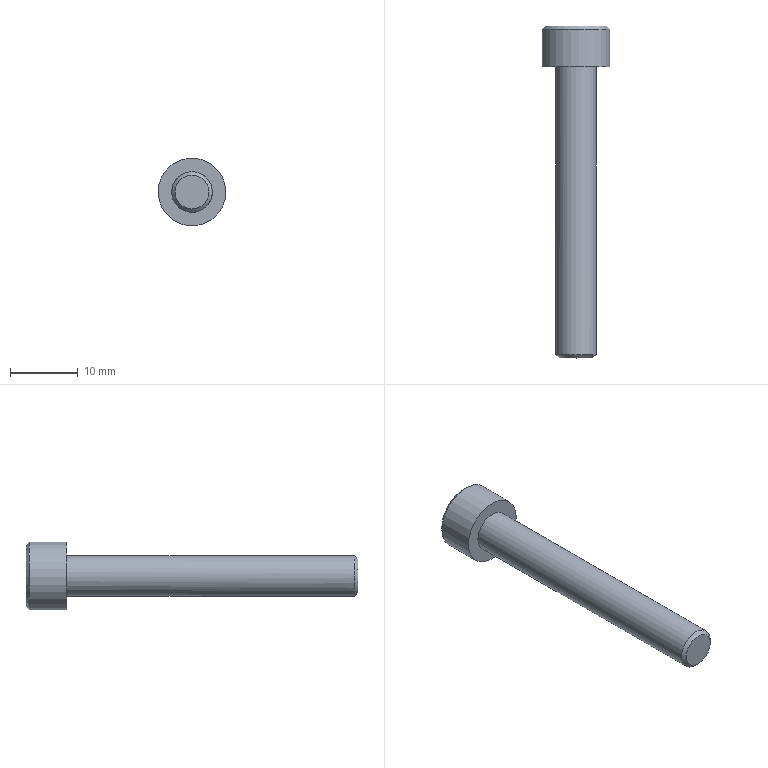Part | NX | features 切除-拉伸1 2 | 1 solid | 20 faces | box 10 x 49 x 10 mm | volume 1607 mm3 | plane 15 | cone 3 | cylinder 2 | commonest cylinder face diameters 6 x1 10 x1
STEP:
#1=CARTESIAN_POINT('',(17.5,309.216,107.881));
#2=VERTEX_POINT('',#1);
#3=CARTESIAN_POINT('',(17.5,309.216,105.381));
#4=DIRECTION('',(0.,1.,0.));
#5=DIRECTION('',(0.,0.,1.));
#6=AXIS2_PLACEMENT_3D('',#3,#4,#5);
#7=CIRCLE('',#6,2.5);
#8=EDGE_CURVE('',#2,#2,#7,.F.);
#9=ORIENTED_EDGE('',*,*,#8,.T.);
#10=EDGE_LOOP('',(#9));
#11=FACE_BOUND('',#10,.T.);
#12=CARTESIAN_POINT('',(-17.5,309.216,105.381));
#13=DIRECTION('',(0.,1.,0.));
#14=DIRECTION('',(-0.07719,0.,0.997));
#15=AXIS2_PLACEMENT_3D('',#12,#13,#14);
#16=PLANE('',#15);
#17=ADVANCED_FACE('',(#11),#16,.F.);
#18=CARTESIAN_POINT('',(17.5,309.716,108.381));
#19=VERTEX_POINT('',#18);
#20=CARTESIAN_POINT('',(17.5,309.716,105.381));
#21=DIRECTION('',(0.,1.,0.));
#22=DIRECTION('',(0.,0.,1.));
#23=AXIS2_PLACEMENT_3D('',#20,#21,#22);
#24=CIRCLE('',#23,3.);
#25=EDGE_CURVE('',#19,#19,#24,.T.);
#26=ORIENTED_EDGE('',*,*,#25,.T.);
#27=EDGE_LOOP('',(#26));
#28=FACE_BOUND('',#27,.T.);
#29=CARTESIAN_POINT('',(14.603,352.216,104.603));
#30=VERTEX_POINT('',#29);
#31=CARTESIAN_POINT('',(17.5,352.216,105.381));
#32=DIRECTION('',(0.,1.,0.));
#33=DIRECTION('',(-0.9657,0.,-0.2595));
#34=AXIS2_PLACEMENT_3D('',#31,#32,#33);
#35=CIRCLE('',#34,3.);
#36=EDGE_CURVE('',#30,#30,#35,.T.);
#37=ORIENTED_EDGE('',*,*,#36,.F.);
#38=EDGE_LOOP('',(#37));
#39=FACE_BOUND('',#38,.T.);
#40=CARTESIAN_POINT('',(17.5,359.966,105.381));
#41=DIRECTION('',(0.,1.,0.));
#42=DIRECTION('',(0.9657,0.,0.2595));
#43=AXIS2_PLACEMENT_3D('',#40,#41,#42);
#44=CYLINDRICAL_SURFACE('',#43,3.);
#45=ADVANCED_FACE('',(#28,#39),#44,.T.);
#46=CARTESIAN_POINT('',(16.855,355.216,102.966));
#47=VERTEX_POINT('',#46);
#48=CARTESIAN_POINT('',(15.086,355.216,104.732));
#49=VERTEX_POINT('',#48);
#50=CARTESIAN_POINT('',(17.5,355.216,105.381));
#51=DIRECTION('',(0.,1.,0.));
#52=DIRECTION('',(-0.9657,0.,-0.2595));
#53=AXIS2_PLACEMENT_3D('',#50,#51,#52);
#54=CIRCLE('',#53,2.5);
#55=EDGE_CURVE('',#47,#49,#54,.T.);
#56=ORIENTED_EDGE('',*,*,#55,.T.);
#57=CARTESIAN_POINT('',(15.731,355.216,107.148));
#58=VERTEX_POINT('',#57);
#59=CARTESIAN_POINT('',(17.5,355.216,105.381));
#60=DIRECTION('',(0.,1.,0.));
#61=DIRECTION('',(-0.9657,0.,-0.2595));
#62=AXIS2_PLACEMENT_3D('',#59,#60,#61);
#63=CIRCLE('',#62,2.5);
#64=EDGE_CURVE('',#49,#58,#63,.T.);
#65=ORIENTED_EDGE('',*,*,#64,.T.);
#66=CARTESIAN_POINT('',(18.145,355.216,107.797));
#67=VERTEX_POINT('',#66);
#68=CARTESIAN_POINT('',(17.5,355.216,105.381));
#69=DIRECTION('',(0.,1.,0.));
#70=DIRECTION('',(-0.9657,0.,-0.2595));
#71=AXIS2_PLACEMENT_3D('',#68,#69,#70);
#72=CIRCLE('',#71,2.5);
#73=EDGE_CURVE('',#58,#67,#72,.T.);
#74=ORIENTED_EDGE('',*,*,#73,.T.);
#75=CARTESIAN_POINT('',(19.914,355.216,106.03));
#76=VERTEX_POINT('',#75);
#77=CARTESIAN_POINT('',(17.5,355.216,105.381));
#78=DIRECTION('',(0.,1.,0.));
#79=DIRECTION('',(-0.9657,0.,-0.2595));
#80=AXIS2_PLACEMENT_3D('',#77,#78,#79);
#81=CIRCLE('',#80,2.5);
#82=EDGE_CURVE('',#67,#76,#81,.T.);
#83=ORIENTED_EDGE('',*,*,#82,.T.);
#84=CARTESIAN_POINT('',(19.269,355.216,103.615));
#85=VERTEX_POINT('',#84);
#86=CARTESIAN_POINT('',(17.5,355.216,105.381));
#87=DIRECTION('',(0.,1.,0.));
#88=DIRECTION('',(-0.9657,0.,-0.2595));
#89=AXIS2_PLACEMENT_3D('',#86,#87,#88);
#90=CIRCLE('',#89,2.5);
#91=EDGE_CURVE('',#76,#85,#90,.T.);
#92=ORIENTED_EDGE('',*,*,#91,.T.);
#93=CARTESIAN_POINT('',(17.5,355.216,105.381));
#94=DIRECTION('',(0.,1.,0.));
#95=DIRECTION('',(-0.9657,0.,-0.2595));
#96=AXIS2_PLACEMENT_3D('',#93,#94,#95);
#97=CIRCLE('',#96,2.5);
#98=EDGE_CURVE('',#85,#47,#97,.T.);
#99=ORIENTED_EDGE('',*,*,#98,.T.);
#100=EDGE_LOOP('',(#56,#65,#74,#83,#92,#99));
#101=FACE_BOUND('',#100,.T.);
#102=CARTESIAN_POINT('',(17.5,353.772,105.381));
#103=VERTEX_POINT('',#102);
#104=VERTEX_LOOP('',#103);
#105=FACE_BOUND('',#104,.T.);
#106=CARTESIAN_POINT('',(17.5,355.216,105.381));
#107=DIRECTION('',(0.,1.,0.));
#108=DIRECTION('',(0.9657,0.,0.2595));
#109=AXIS2_PLACEMENT_3D('',#106,#107,#108);
#110=CONICAL_SURFACE('',#109,2.5,1.047);
#111=ADVANCED_FACE('',(#101,#105),#110,.F.);
#112=CARTESIAN_POINT('',(22.329,357.736,106.679));
#113=VERTEX_POINT('',#112);
#114=CARTESIAN_POINT('',(17.5,357.736,105.381));
#115=DIRECTION('',(0.,-1.,0.));
#116=DIRECTION('',(0.9657,0.,0.2595));
#117=AXIS2_PLACEMENT_3D('',#114,#115,#116);
#118=CIRCLE('',#117,5.);
#119=EDGE_CURVE('',#113,#113,#118,.T.);
#120=ORIENTED_EDGE('',*,*,#119,.F.);
#121=EDGE_LOOP('',(#120));
#122=FACE_BOUND('',#121,.T.);
#123=CARTESIAN_POINT('',(21.865,358.216,106.554));
#124=VERTEX_POINT('',#123);
#125=CARTESIAN_POINT('',(17.5,358.216,105.381));
#126=DIRECTION('',(0.,1.,0.));
#127=DIRECTION('',(0.9657,0.,0.2595));
#128=AXIS2_PLACEMENT_3D('',#125,#126,#127);
#129=CIRCLE('',#128,4.52);
#130=EDGE_CURVE('',#124,#124,#129,.T.);
#131=ORIENTED_EDGE('',*,*,#130,.F.);
#132=EDGE_LOOP('',(#131));
#133=FACE_BOUND('',#132,.T.);
#134=CARTESIAN_POINT('',(17.5,358.216,105.381));
#135=DIRECTION('',(0.,-1.,0.));
#136=DIRECTION('',(-0.9657,0.,-0.2595));
#137=AXIS2_PLACEMENT_3D('',#134,#135,#136);
#138=CONICAL_SURFACE('',#137,4.52,0.7854);
#139=ADVANCED_FACE('',(#122,#133),#138,.T.);
#140=ORIENTED_EDGE('',*,*,#119,.T.);
#141=EDGE_LOOP('',(#140));
#142=FACE_BOUND('',#141,.T.);
#143=CARTESIAN_POINT('',(12.671,352.216,104.083));
#144=VERTEX_POINT('',#143);
#145=CARTESIAN_POINT('',(17.5,352.216,105.381));
#146=DIRECTION('',(0.,1.,0.));
#147=DIRECTION('',(-0.9657,0.,-0.2595));
#148=AXIS2_PLACEMENT_3D('',#145,#146,#147);
#149=CIRCLE('',#148,5.);
#150=EDGE_CURVE('',#144,#144,#149,.T.);
#151=ORIENTED_EDGE('',*,*,#150,.T.);
#152=EDGE_LOOP('',(#151));
#153=FACE_BOUND('',#152,.T.);
#154=CARTESIAN_POINT('',(17.5,359.966,105.381));
#155=DIRECTION('',(0.,1.,0.));
#156=DIRECTION('',(0.9657,0.,0.2595));
#157=AXIS2_PLACEMENT_3D('',#154,#155,#156);
#158=CYLINDRICAL_SURFACE('',#157,5.);
#159=ADVANCED_FACE('',(#142,#153),#158,.T.);
#160=ORIENTED_EDGE('',*,*,#130,.T.);
#161=EDGE_LOOP('',(#160));
#162=FACE_BOUND('',#161,.T.);
#163=CARTESIAN_POINT('',(19.54,358.216,107.424));
#164=VERTEX_POINT('',#163);
#165=CARTESIAN_POINT('',(16.751,358.216,108.169));
#166=VERTEX_POINT('',#165);
#167=CARTESIAN_POINT('',(20.237,358.216,107.238));
#168=DIRECTION('',(-0.9661,0.,0.2581));
#169=VECTOR('',#168,1000.);
#170=LINE('',#167,#169);
#171=EDGE_CURVE('',#164,#166,#170,.T.);
#172=ORIENTED_EDGE('',*,*,#171,.T.);
#173=CARTESIAN_POINT('',(14.711,358.216,106.126));
#174=VERTEX_POINT('',#173);
#175=CARTESIAN_POINT('',(17.261,358.216,108.68));
#176=DIRECTION('',(-0.7066,0.,-0.7076));
#177=VECTOR('',#176,1000.);
#178=LINE('',#175,#177);
#179=EDGE_CURVE('',#166,#174,#178,.T.);
#180=ORIENTED_EDGE('',*,*,#179,.T.);
#181=CARTESIAN_POINT('',(15.46,358.216,103.338));
#182=VERTEX_POINT('',#181);
#183=CARTESIAN_POINT('',(15.086,358.216,104.732));
#184=DIRECTION('',(0.2595,0.,-0.9657));
#185=VECTOR('',#184,1000.);
#186=LINE('',#183,#185);
#187=EDGE_CURVE('',#174,#182,#186,.T.);
#188=ORIENTED_EDGE('',*,*,#187,.T.);
#189=CARTESIAN_POINT('',(18.249,358.216,102.593));
#190=VERTEX_POINT('',#189);
#191=CARTESIAN_POINT('',(18.946,358.216,102.407));
#192=DIRECTION('',(0.9661,0.,-0.2581));
#193=VECTOR('',#192,1000.);
#194=LINE('',#191,#193);
#195=EDGE_CURVE('',#182,#190,#194,.T.);
#196=ORIENTED_EDGE('',*,*,#195,.T.);
#197=CARTESIAN_POINT('',(20.289,358.216,104.636));
#198=VERTEX_POINT('',#197);
#199=CARTESIAN_POINT('',(20.799,358.216,105.147));
#200=DIRECTION('',(0.7066,0.,0.7076));
#201=VECTOR('',#200,1000.);
#202=LINE('',#199,#201);
#203=EDGE_CURVE('',#190,#198,#202,.T.);
#204=ORIENTED_EDGE('',*,*,#203,.T.);
#205=CARTESIAN_POINT('',(19.914,358.216,106.03));
#206=DIRECTION('',(-0.2595,0.,0.9657));
#207=VECTOR('',#206,1000.);
#208=LINE('',#205,#207);
#209=EDGE_CURVE('',#198,#164,#208,.T.);
#210=ORIENTED_EDGE('',*,*,#209,.T.);
#211=EDGE_LOOP('',(#172,#180,#188,#196,#204,#210));
#212=FACE_BOUND('',#211,.T.);
#213=CARTESIAN_POINT('',(19.914,358.216,106.03));
#214=DIRECTION('',(0.,-1.,0.));
#215=DIRECTION('',(-0.9657,0.,-0.2595));
#216=AXIS2_PLACEMENT_3D('',#213,#214,#215);
#217=PLANE('',#216);
#218=ADVANCED_FACE('',(#162,#212),#217,.F.);
#219=ORIENTED_EDGE('',*,*,#150,.F.);
#220=EDGE_LOOP('',(#219));
#221=FACE_BOUND('',#220,.T.);
#222=ORIENTED_EDGE('',*,*,#36,.T.);
#223=EDGE_LOOP('',(#222));
#224=FACE_BOUND('',#223,.T.);
#225=CARTESIAN_POINT('',(22.329,352.216,106.679));
#226=DIRECTION('',(0.,1.,0.));
#227=DIRECTION('',(0.9657,0.,0.2595));
#228=AXIS2_PLACEMENT_3D('',#225,#226,#227);
#229=PLANE('',#228);
#230=ADVANCED_FACE('',(#221,#224),#229,.F.);
#231=ORIENTED_EDGE('',*,*,#64,.F.);
#232=CARTESIAN_POINT('',(14.711,355.216,106.126));
#233=VERTEX_POINT('',#232);
#234=CARTESIAN_POINT('',(15.46,355.216,103.338));
#235=DIRECTION('',(-0.2595,0.,0.9657));
#236=VECTOR('',#235,1000.);
#237=LINE('',#234,#236);
#238=EDGE_CURVE('',#49,#233,#237,.T.);
#239=ORIENTED_EDGE('',*,*,#238,.T.);
#240=CARTESIAN_POINT('',(14.711,355.216,106.126));
#241=DIRECTION('',(0.7066,0.,0.7076));
#242=VECTOR('',#241,1000.);
#243=LINE('',#240,#242);
#244=EDGE_CURVE('',#233,#58,#243,.T.);
#245=ORIENTED_EDGE('',*,*,#244,.T.);
#246=EDGE_LOOP('',(#231,#239,#245));
#247=FACE_BOUND('',#246,.T.);
#248=CARTESIAN_POINT('',(17.5,355.216,105.381));
#249=DIRECTION('',(0.,1.,0.));
#250=DIRECTION('',(0.2595,0.,-0.9657));
#251=AXIS2_PLACEMENT_3D('',#248,#249,#250);
#252=PLANE('',#251);
#253=ADVANCED_FACE('',(#247),#252,.T.);
#254=ORIENTED_EDGE('',*,*,#55,.F.);
#255=CARTESIAN_POINT('',(15.46,355.216,103.338));
#256=VERTEX_POINT('',#255);
#257=CARTESIAN_POINT('',(18.249,355.216,102.593));
#258=DIRECTION('',(-0.9661,0.,0.2581));
#259=VECTOR('',#258,1000.);
#260=LINE('',#257,#259);
#261=EDGE_CURVE('',#47,#256,#260,.T.);
#262=ORIENTED_EDGE('',*,*,#261,.T.);
#263=CARTESIAN_POINT('',(15.46,355.216,103.338));
#264=DIRECTION('',(-0.2595,0.,0.9657));
#265=VECTOR('',#264,1000.);
#266=LINE('',#263,#265);
#267=EDGE_CURVE('',#256,#49,#266,.T.);
#268=ORIENTED_EDGE('',*,*,#267,.T.);
#269=EDGE_LOOP('',(#254,#262,#268));
#270=FACE_BOUND('',#269,.T.);
#271=CARTESIAN_POINT('',(17.5,355.216,105.381));
#272=DIRECTION('',(0.,1.,0.));
#273=DIRECTION('',(0.2595,0.,-0.9657));
#274=AXIS2_PLACEMENT_3D('',#271,#272,#273);
#275=PLANE('',#274);
#276=ADVANCED_FACE('',(#270),#275,.T.);
#277=ORIENTED_EDGE('',*,*,#98,.F.);
#278=CARTESIAN_POINT('',(18.249,355.216,102.593));
#279=VERTEX_POINT('',#278);
#280=CARTESIAN_POINT('',(20.289,355.216,104.636));
#281=DIRECTION('',(-0.7066,0.,-0.7076));
#282=VECTOR('',#281,1000.);
#283=LINE('',#280,#282);
#284=EDGE_CURVE('',#85,#279,#283,.T.);
#285=ORIENTED_EDGE('',*,*,#284,.T.);
#286=CARTESIAN_POINT('',(18.249,355.216,102.593));
#287=DIRECTION('',(-0.9661,0.,0.2581));
#288=VECTOR('',#287,1000.);
#289=LINE('',#286,#288);
#290=EDGE_CURVE('',#279,#47,#289,.T.);
#291=ORIENTED_EDGE('',*,*,#290,.T.);
#292=EDGE_LOOP('',(#277,#285,#291));
#293=FACE_BOUND('',#292,.T.);
#294=CARTESIAN_POINT('',(17.5,355.216,105.381));
#295=DIRECTION('',(0.,1.,0.));
#296=DIRECTION('',(0.2595,0.,-0.9657));
#297=AXIS2_PLACEMENT_3D('',#294,#295,#296);
#298=PLANE('',#297);
#299=ADVANCED_FACE('',(#293),#298,.T.);
#300=ORIENTED_EDGE('',*,*,#91,.F.);
#301=CARTESIAN_POINT('',(20.289,355.216,104.636));
#302=VERTEX_POINT('',#301);
#303=CARTESIAN_POINT('',(19.54,355.216,107.424));
#304=DIRECTION('',(0.2595,0.,-0.9657));
#305=VECTOR('',#304,1000.);
#306=LINE('',#303,#305);
#307=EDGE_CURVE('',#76,#302,#306,.T.);
#308=ORIENTED_EDGE('',*,*,#307,.T.);
#309=CARTESIAN_POINT('',(20.289,355.216,104.636));
#310=DIRECTION('',(-0.7066,0.,-0.7076));
#311=VECTOR('',#310,1000.);
#312=LINE('',#309,#311);
#313=EDGE_CURVE('',#302,#85,#312,.T.);
#314=ORIENTED_EDGE('',*,*,#313,.T.);
#315=EDGE_LOOP('',(#300,#308,#314));
#316=FACE_BOUND('',#315,.T.);
#317=CARTESIAN_POINT('',(17.5,355.216,105.381));
#318=DIRECTION('',(0.,1.,0.));
#319=DIRECTION('',(0.2595,0.,-0.9657));
#320=AXIS2_PLACEMENT_3D('',#317,#318,#319);
#321=PLANE('',#320);
#322=ADVANCED_FACE('',(#316),#321,.T.);
#323=ORIENTED_EDGE('',*,*,#82,.F.);
#324=CARTESIAN_POINT('',(19.54,355.216,107.424));
#325=VERTEX_POINT('',#324);
#326=CARTESIAN_POINT('',(16.751,355.216,108.169));
#327=DIRECTION('',(0.9661,0.,-0.2581));
#328=VECTOR('',#327,1000.);
#329=LINE('',#326,#328);
#330=EDGE_CURVE('',#67,#325,#329,.T.);
#331=ORIENTED_EDGE('',*,*,#330,.T.);
#332=CARTESIAN_POINT('',(19.54,355.216,107.424));
#333=DIRECTION('',(0.2595,0.,-0.9657));
#334=VECTOR('',#333,1000.);
#335=LINE('',#332,#334);
#336=EDGE_CURVE('',#325,#76,#335,.T.);
#337=ORIENTED_EDGE('',*,*,#336,.T.);
#338=EDGE_LOOP('',(#323,#331,#337));
#339=FACE_BOUND('',#338,.T.);
#340=CARTESIAN_POINT('',(17.5,355.216,105.381));
#341=DIRECTION('',(0.,1.,0.));
#342=DIRECTION('',(0.2595,0.,-0.9657));
#343=AXIS2_PLACEMENT_3D('',#340,#341,#342);
#344=PLANE('',#343);
#345=ADVANCED_FACE('',(#339),#344,.T.);
#346=ORIENTED_EDGE('',*,*,#73,.F.);
#347=CARTESIAN_POINT('',(16.751,355.216,108.169));
#348=VERTEX_POINT('',#347);
#349=CARTESIAN_POINT('',(14.711,355.216,106.126));
#350=DIRECTION('',(0.7066,0.,0.7076));
#351=VECTOR('',#350,1000.);
#352=LINE('',#349,#351);
#353=EDGE_CURVE('',#58,#348,#352,.T.);
#354=ORIENTED_EDGE('',*,*,#353,.T.);
#355=CARTESIAN_POINT('',(16.751,355.216,108.169));
#356=DIRECTION('',(0.9661,0.,-0.2581));
#357=VECTOR('',#356,1000.);
#358=LINE('',#355,#357);
#359=EDGE_CURVE('',#348,#67,#358,.T.);
#360=ORIENTED_EDGE('',*,*,#359,.T.);
#361=EDGE_LOOP('',(#346,#354,#360));
#362=FACE_BOUND('',#361,.T.);
#363=CARTESIAN_POINT('',(17.5,355.216,105.381));
#364=DIRECTION('',(0.,1.,0.));
#365=DIRECTION('',(0.2595,0.,-0.9657));
#366=AXIS2_PLACEMENT_3D('',#363,#364,#365);
#367=PLANE('',#366);
#368=ADVANCED_FACE('',(#362),#367,.T.);
#369=ORIENTED_EDGE('',*,*,#179,.F.);
#370=CARTESIAN_POINT('',(16.751,355.216,108.169));
#371=DIRECTION('',(0.,1.,0.));
#372=VECTOR('',#371,1000.);
#373=LINE('',#370,#372);
#374=EDGE_CURVE('',#348,#166,#373,.T.);
#375=ORIENTED_EDGE('',*,*,#374,.F.);
#376=ORIENTED_EDGE('',*,*,#353,.F.);
#377=ORIENTED_EDGE('',*,*,#244,.F.);
#378=CARTESIAN_POINT('',(14.711,355.216,106.126));
#379=DIRECTION('',(0.,1.,0.));
#380=VECTOR('',#379,1000.);
#381=LINE('',#378,#380);
#382=EDGE_CURVE('',#233,#174,#381,.T.);
#383=ORIENTED_EDGE('',*,*,#382,.T.);
#384=EDGE_LOOP('',(#369,#375,#376,#377,#383));
#385=FACE_BOUND('',#384,.T.);
#386=CARTESIAN_POINT('',(14.711,355.216,106.126));
#387=DIRECTION('',(-0.7076,0.,0.7066));
#388=DIRECTION('',(0.7066,0.,0.7076));
#389=AXIS2_PLACEMENT_3D('',#386,#387,#388);
#390=PLANE('',#389);
#391=ADVANCED_FACE('',(#385),#390,.F.);
#392=ORIENTED_EDGE('',*,*,#187,.F.);
#393=ORIENTED_EDGE('',*,*,#382,.F.);
#394=ORIENTED_EDGE('',*,*,#238,.F.);
#395=ORIENTED_EDGE('',*,*,#267,.F.);
#396=CARTESIAN_POINT('',(15.46,355.216,103.338));
#397=DIRECTION('',(0.,1.,0.));
#398=VECTOR('',#397,1000.);
#399=LINE('',#396,#398);
#400=EDGE_CURVE('',#256,#182,#399,.T.);
#401=ORIENTED_EDGE('',*,*,#400,.T.);
#402=EDGE_LOOP('',(#392,#393,#394,#395,#401));
#403=FACE_BOUND('',#402,.T.);
#404=CARTESIAN_POINT('',(15.46,355.216,103.338));
#405=DIRECTION('',(-0.9657,0.,-0.2595));
#406=DIRECTION('',(0.,1.,0.));
#407=AXIS2_PLACEMENT_3D('',#404,#405,#406);
#408=PLANE('',#407);
#409=ADVANCED_FACE('',(#403),#408,.F.);
#410=ORIENTED_EDGE('',*,*,#195,.F.);
#411=ORIENTED_EDGE('',*,*,#400,.F.);
#412=ORIENTED_EDGE('',*,*,#261,.F.);
#413=ORIENTED_EDGE('',*,*,#290,.F.);
#414=CARTESIAN_POINT('',(18.249,355.216,102.593));
#415=DIRECTION('',(0.,1.,0.));
#416=VECTOR('',#415,1000.);
#417=LINE('',#414,#416);
#418=EDGE_CURVE('',#279,#190,#417,.T.);
#419=ORIENTED_EDGE('',*,*,#418,.T.);
#420=EDGE_LOOP('',(#410,#411,#412,#413,#419));
#421=FACE_BOUND('',#420,.T.);
#422=CARTESIAN_POINT('',(18.249,355.216,102.593));
#423=DIRECTION('',(-0.2581,0.,-0.9661));
#424=DIRECTION('',(-0.9661,0.,0.2581));
#425=AXIS2_PLACEMENT_3D('',#422,#423,#424);
#426=PLANE('',#425);
#427=ADVANCED_FACE('',(#421),#426,.F.);
#428=ORIENTED_EDGE('',*,*,#203,.F.);
#429=ORIENTED_EDGE('',*,*,#418,.F.);
#430=ORIENTED_EDGE('',*,*,#284,.F.);
#431=ORIENTED_EDGE('',*,*,#313,.F.);
#432=CARTESIAN_POINT('',(20.289,355.216,104.636));
#433=DIRECTION('',(0.,1.,0.));
#434=VECTOR('',#433,1000.);
#435=LINE('',#432,#434);
#436=EDGE_CURVE('',#302,#198,#435,.T.);
#437=ORIENTED_EDGE('',*,*,#436,.T.);
#438=EDGE_LOOP('',(#428,#429,#430,#431,#437));
#439=FACE_BOUND('',#438,.T.);
#440=CARTESIAN_POINT('',(20.289,355.216,104.636));
#441=DIRECTION('',(0.7076,0.,-0.7066));
#442=DIRECTION('',(-0.7066,0.,-0.7076));
#443=AXIS2_PLACEMENT_3D('',#440,#441,#442);
#444=PLANE('',#443);
#445=ADVANCED_FACE('',(#439),#444,.F.);
#446=ORIENTED_EDGE('',*,*,#209,.F.);
#447=ORIENTED_EDGE('',*,*,#436,.F.);
#448=ORIENTED_EDGE('',*,*,#307,.F.);
#449=ORIENTED_EDGE('',*,*,#336,.F.);
#450=CARTESIAN_POINT('',(19.54,355.216,107.424));
#451=DIRECTION('',(0.,1.,0.));
#452=VECTOR('',#451,1000.);
#453=LINE('',#450,#452);
#454=EDGE_CURVE('',#325,#164,#453,.T.);
#455=ORIENTED_EDGE('',*,*,#454,.T.);
#456=EDGE_LOOP('',(#446,#447,#448,#449,#455));
#457=FACE_BOUND('',#456,.T.);
#458=CARTESIAN_POINT('',(19.54,355.216,107.424));
#459=DIRECTION('',(0.9657,0.,0.2595));
#460=DIRECTION('',(0.,-1.,0.));
#461=AXIS2_PLACEMENT_3D('',#458,#459,#460);
#462=PLANE('',#461);
#463=ADVANCED_FACE('',(#457),#462,.F.);
#464=ORIENTED_EDGE('',*,*,#171,.F.);
#465=ORIENTED_EDGE('',*,*,#454,.F.);
#466=ORIENTED_EDGE('',*,*,#330,.F.);
#467=ORIENTED_EDGE('',*,*,#359,.F.);
#468=ORIENTED_EDGE('',*,*,#374,.T.);
#469=EDGE_LOOP('',(#464,#465,#466,#467,#468));
#470=FACE_BOUND('',#469,.T.);
#471=CARTESIAN_POINT('',(16.751,355.216,108.169));
#472=DIRECTION('',(0.2581,0.,0.9661));
#473=DIRECTION('',(0.9661,0.,-0.2581));
#474=AXIS2_PLACEMENT_3D('',#471,#472,#473);
#475=PLANE('',#474);
#476=ADVANCED_FACE('',(#470),#475,.F.);
#477=ORIENTED_EDGE('',*,*,#8,.F.);
#478=EDGE_LOOP('',(#477));
#479=FACE_BOUND('',#478,.T.);
#480=ORIENTED_EDGE('',*,*,#25,.F.);
#481=EDGE_LOOP('',(#480));
#482=FACE_BOUND('',#481,.T.);
#483=CARTESIAN_POINT('',(17.5,309.716,105.381));
#484=DIRECTION('',(0.,1.,0.));
#485=DIRECTION('',(0.,0.,1.));
#486=AXIS2_PLACEMENT_3D('',#483,#484,#485);
#487=CONICAL_SURFACE('',#486,3.,0.7854);
#488=ADVANCED_FACE('',(#479,#482),#487,.T.);
#489=CLOSED_SHELL('',(#17,#45,#111,#139,#159,#218,#230,#253,#276,#299,#322,#345,#368,#391,#409,#427,#445,#463,#476,#488));
#490=MANIFOLD_SOLID_BREP('',#489);
#491=(LENGTH_UNIT()NAMED_UNIT(*)SI_UNIT(.MILLI.,.METRE.));
#492=UNCERTAINTY_MEASURE_WITH_UNIT(LENGTH_MEASURE(0.00001),#491,'','');
#493=(NAMED_UNIT(*)PLANE_ANGLE_UNIT()SI_UNIT($,.RADIAN.));
#494=(NAMED_UNIT(*)SI_UNIT($,.STERADIAN.)SOLID_ANGLE_UNIT());
#495=(GEOMETRIC_REPRESENTATION_CONTEXT(3)GLOBAL_UNCERTAINTY_ASSIGNED_CONTEXT((#492))GLOBAL_UNIT_ASSIGNED_CONTEXT((#491,#493,#494))REPRESENTATION_CONTEXT('',''));
#496=ADVANCED_BREP_SHAPE_REPRESENTATION('',(#490),#495);